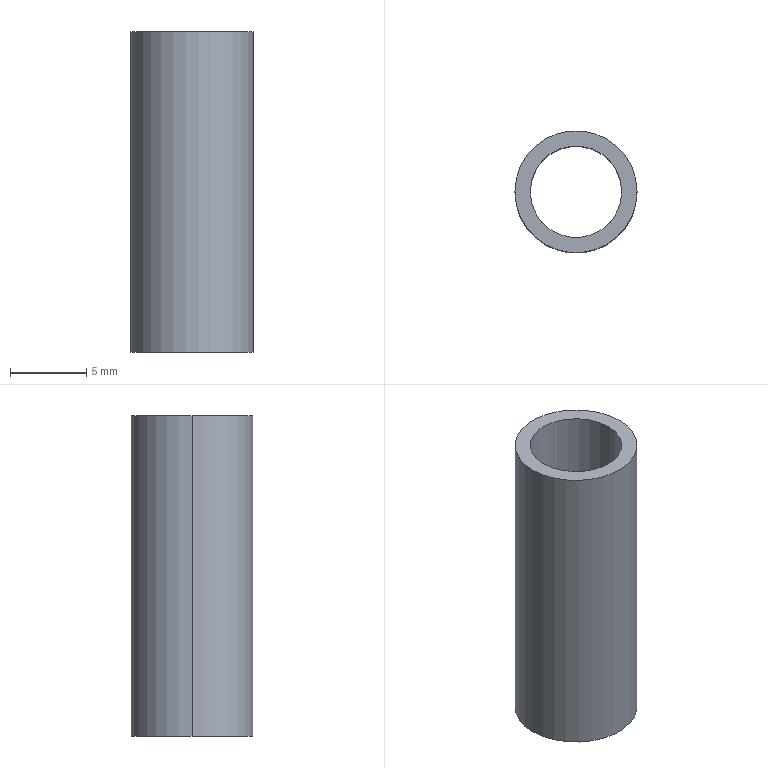Part | STEP file | PN_0001 Wheel body | 1 solid | 6 faces | box 8 x 8 x 21 mm | volume 461.814 mm3 | cylinder 4 | plane 2 | commonest cylinder face diameters 6 x2 8 x2
STEP:
#1=CARTESIAN_POINT('',(0.,0.,0.));
#2=DIRECTION('',(0.,0.,1.));
#3=DIRECTION('',(1.,0.,0.));
#4=AXIS2_PLACEMENT_3D('',#1,#2,#3);
#5=CARTESIAN_POINT('',(20.,-37.5,10.5));
#6=VERTEX_POINT('',#5);
#7=CARTESIAN_POINT('',(20.,-37.5,-10.5));
#8=VERTEX_POINT('',#7);
#9=CARTESIAN_POINT('',(20.,-37.5,10.5));
#10=DIRECTION('',(0.,0.,-1.));
#11=VECTOR('',#10,1.);
#12=LINE('',#9,#11);
#13=CARTESIAN_POINT('',(23.,-37.5,10.5));
#14=DIRECTION('',(0.,0.,-1.));
#15=DIRECTION('',(-1.,0.,0.));
#16=AXIS2_PLACEMENT_3D('',#13,#14,#15);
#17=CYLINDRICAL_SURFACE('',#16,3.);
#18=CARTESIAN_POINT('',(6.283,0.));
#19=DIRECTION('',(0.,1.));
#20=VECTOR('',#19,1.);
#21=LINE('',#18,#20);
#22=(GEOMETRIC_REPRESENTATION_CONTEXT(2)PARAMETRIC_REPRESENTATION_CONTEXT()REPRESENTATION_CONTEXT('',''));
#23=DEFINITIONAL_REPRESENTATION('',(#21),#22);
#24=PCURVE('',#17,#23);
#25=CARTESIAN_POINT('',(23.,-37.5,10.5));
#26=DIRECTION('',(0.,0.,-1.));
#27=DIRECTION('',(-1.,0.,0.));
#28=AXIS2_PLACEMENT_3D('',#25,#26,#27);
#29=CYLINDRICAL_SURFACE('',#28,3.);
#30=CARTESIAN_POINT('',(0.,0.));
#31=DIRECTION('',(0.,1.));
#32=VECTOR('',#31,1.);
#33=LINE('',#30,#32);
#34=(GEOMETRIC_REPRESENTATION_CONTEXT(2)PARAMETRIC_REPRESENTATION_CONTEXT()REPRESENTATION_CONTEXT('',''));
#35=DEFINITIONAL_REPRESENTATION('',(#33),#34);
#36=PCURVE('',#29,#35);
#37=SURFACE_CURVE('',#12,(#24,#36),.PCURVE_S1.);
#38=EDGE_CURVE('',#6,#8,#37,.T.);
#39=ORIENTED_EDGE('',*,*,#38,.T.);
#40=CARTESIAN_POINT('',(26.,-37.5,-10.5));
#41=VERTEX_POINT('',#40);
#42=CARTESIAN_POINT('',(23.,-37.5,-10.5));
#43=DIRECTION('',(0.,0.,1.));
#44=DIRECTION('',(1.,0.,0.));
#45=AXIS2_PLACEMENT_3D('',#42,#43,#44);
#46=CIRCLE('',#45,3.);
#47=CARTESIAN_POINT('',(9.425,21.));
#48=DIRECTION('',(-1.,0.));
#49=VECTOR('',#48,1.);
#50=LINE('',#47,#49);
#51=(GEOMETRIC_REPRESENTATION_CONTEXT(2)PARAMETRIC_REPRESENTATION_CONTEXT()REPRESENTATION_CONTEXT('',''));
#52=DEFINITIONAL_REPRESENTATION('',(#50),#51);
#53=PCURVE('',#17,#52);
#54=CARTESIAN_POINT('',(23.,-37.5,-10.5));
#55=DIRECTION('',(0.,0.,1.));
#56=DIRECTION('',(1.,0.,0.));
#57=AXIS2_PLACEMENT_3D('',#54,#55,#56);
#58=PLANE('',#57);
#59=CARTESIAN_POINT('',(0.,0.));
#60=DIRECTION('',(1.,0.));
#61=AXIS2_PLACEMENT_2D('',#59,#60);
#62=CIRCLE('',#61,3.);
#63=(GEOMETRIC_REPRESENTATION_CONTEXT(2)PARAMETRIC_REPRESENTATION_CONTEXT()REPRESENTATION_CONTEXT('',''));
#64=DEFINITIONAL_REPRESENTATION('',(#62),#63);
#65=PCURVE('',#58,#64);
#66=SURFACE_CURVE('',#46,(#53,#65),.PCURVE_S1.);
#67=EDGE_CURVE('',#8,#41,#66,.T.);
#68=ORIENTED_EDGE('',*,*,#67,.T.);
#69=CARTESIAN_POINT('',(26.,-37.5,10.5));
#70=VERTEX_POINT('',#69);
#71=CARTESIAN_POINT('',(26.,-37.5,10.5));
#72=DIRECTION('',(0.,0.,-1.));
#73=VECTOR('',#72,1.);
#74=LINE('',#71,#73);
#75=CARTESIAN_POINT('',(3.142,0.));
#76=DIRECTION('',(0.,1.));
#77=VECTOR('',#76,1.);
#78=LINE('',#75,#77);
#79=(GEOMETRIC_REPRESENTATION_CONTEXT(2)PARAMETRIC_REPRESENTATION_CONTEXT()REPRESENTATION_CONTEXT('',''));
#80=DEFINITIONAL_REPRESENTATION('',(#78),#79);
#81=PCURVE('',#17,#80);
#82=CARTESIAN_POINT('',(3.142,0.));
#83=DIRECTION('',(0.,1.));
#84=VECTOR('',#83,1.);
#85=LINE('',#82,#84);
#86=(GEOMETRIC_REPRESENTATION_CONTEXT(2)PARAMETRIC_REPRESENTATION_CONTEXT()REPRESENTATION_CONTEXT('',''));
#87=DEFINITIONAL_REPRESENTATION('',(#85),#86);
#88=PCURVE('',#29,#87);
#89=SURFACE_CURVE('',#74,(#81,#88),.PCURVE_S1.);
#90=EDGE_CURVE('',#70,#41,#89,.T.);
#91=ORIENTED_EDGE('',*,*,#90,.F.);
#92=CARTESIAN_POINT('',(23.,-37.5,10.5));
#93=DIRECTION('',(0.,0.,1.));
#94=DIRECTION('',(1.,0.,0.));
#95=AXIS2_PLACEMENT_3D('',#92,#93,#94);
#96=CIRCLE('',#95,3.);
#97=CARTESIAN_POINT('',(9.425,0.));
#98=DIRECTION('',(-1.,0.));
#99=VECTOR('',#98,1.);
#100=LINE('',#97,#99);
#101=(GEOMETRIC_REPRESENTATION_CONTEXT(2)PARAMETRIC_REPRESENTATION_CONTEXT()REPRESENTATION_CONTEXT('',''));
#102=DEFINITIONAL_REPRESENTATION('',(#100),#101);
#103=PCURVE('',#17,#102);
#104=CARTESIAN_POINT('',(23.,-37.5,10.5));
#105=DIRECTION('',(0.,0.,1.));
#106=DIRECTION('',(1.,0.,0.));
#107=AXIS2_PLACEMENT_3D('',#104,#105,#106);
#108=PLANE('',#107);
#109=CARTESIAN_POINT('',(0.,0.));
#110=DIRECTION('',(1.,0.));
#111=AXIS2_PLACEMENT_2D('',#109,#110);
#112=CIRCLE('',#111,3.);
#113=(GEOMETRIC_REPRESENTATION_CONTEXT(2)PARAMETRIC_REPRESENTATION_CONTEXT()REPRESENTATION_CONTEXT('',''));
#114=DEFINITIONAL_REPRESENTATION('',(#112),#113);
#115=PCURVE('',#108,#114);
#116=SURFACE_CURVE('',#96,(#103,#115),.PCURVE_S1.);
#117=EDGE_CURVE('',#6,#70,#116,.T.);
#118=ORIENTED_EDGE('',*,*,#117,.F.);
#119=EDGE_LOOP('',(#39,#68,#91,#118));
#120=FACE_BOUND('',#119,.F.);
#121=ADVANCED_FACE('',(#120),#17,.F.);
#122=CARTESIAN_POINT('',(27.,-37.5,10.5));
#123=VERTEX_POINT('',#122);
#124=CARTESIAN_POINT('',(19.,-37.5,10.5));
#125=VERTEX_POINT('',#124);
#126=CARTESIAN_POINT('',(23.,-37.5,10.5));
#127=DIRECTION('',(0.,0.,1.));
#128=DIRECTION('',(1.,0.,0.));
#129=AXIS2_PLACEMENT_3D('',#126,#127,#128);
#130=CIRCLE('',#129,4.);
#131=CARTESIAN_POINT('',(23.,-37.5,10.5));
#132=DIRECTION('',(0.,0.,-1.));
#133=DIRECTION('',(-1.,0.,0.));
#134=AXIS2_PLACEMENT_3D('',#131,#132,#133);
#135=CYLINDRICAL_SURFACE('',#134,4.);
#136=CARTESIAN_POINT('',(3.142,0.));
#137=DIRECTION('',(-1.,0.));
#138=VECTOR('',#137,1.);
#139=LINE('',#136,#138);
#140=(GEOMETRIC_REPRESENTATION_CONTEXT(2)PARAMETRIC_REPRESENTATION_CONTEXT()REPRESENTATION_CONTEXT('',''));
#141=DEFINITIONAL_REPRESENTATION('',(#139),#140);
#142=PCURVE('',#135,#141);
#143=CARTESIAN_POINT('',(0.,0.));
#144=DIRECTION('',(1.,0.));
#145=AXIS2_PLACEMENT_2D('',#143,#144);
#146=CIRCLE('',#145,4.);
#147=(GEOMETRIC_REPRESENTATION_CONTEXT(2)PARAMETRIC_REPRESENTATION_CONTEXT()REPRESENTATION_CONTEXT('',''));
#148=DEFINITIONAL_REPRESENTATION('',(#146),#147);
#149=PCURVE('',#108,#148);
#150=SURFACE_CURVE('',#130,(#142,#149),.PCURVE_S1.);
#151=EDGE_CURVE('',#123,#125,#150,.T.);
#152=ORIENTED_EDGE('',*,*,#151,.F.);
#153=CARTESIAN_POINT('',(27.,-37.5,-10.5));
#154=VERTEX_POINT('',#153);
#155=CARTESIAN_POINT('',(27.,-37.5,10.5));
#156=DIRECTION('',(0.,0.,-1.));
#157=VECTOR('',#156,1.);
#158=LINE('',#155,#157);
#159=CARTESIAN_POINT('',(3.142,0.));
#160=DIRECTION('',(0.,1.));
#161=VECTOR('',#160,1.);
#162=LINE('',#159,#161);
#163=(GEOMETRIC_REPRESENTATION_CONTEXT(2)PARAMETRIC_REPRESENTATION_CONTEXT()REPRESENTATION_CONTEXT('',''));
#164=DEFINITIONAL_REPRESENTATION('',(#162),#163);
#165=PCURVE('',#135,#164);
#166=CARTESIAN_POINT('',(23.,-37.5,10.5));
#167=DIRECTION('',(0.,0.,-1.));
#168=DIRECTION('',(-1.,0.,0.));
#169=AXIS2_PLACEMENT_3D('',#166,#167,#168);
#170=CYLINDRICAL_SURFACE('',#169,4.);
#171=CARTESIAN_POINT('',(3.142,0.));
#172=DIRECTION('',(0.,1.));
#173=VECTOR('',#172,1.);
#174=LINE('',#171,#173);
#175=(GEOMETRIC_REPRESENTATION_CONTEXT(2)PARAMETRIC_REPRESENTATION_CONTEXT()REPRESENTATION_CONTEXT('',''));
#176=DEFINITIONAL_REPRESENTATION('',(#174),#175);
#177=PCURVE('',#170,#176);
#178=SURFACE_CURVE('',#158,(#165,#177),.PCURVE_S1.);
#179=EDGE_CURVE('',#123,#154,#178,.T.);
#180=ORIENTED_EDGE('',*,*,#179,.T.);
#181=CARTESIAN_POINT('',(19.,-37.5,-10.5));
#182=VERTEX_POINT('',#181);
#183=CARTESIAN_POINT('',(23.,-37.5,-10.5));
#184=DIRECTION('',(0.,0.,1.));
#185=DIRECTION('',(1.,0.,0.));
#186=AXIS2_PLACEMENT_3D('',#183,#184,#185);
#187=CIRCLE('',#186,4.);
#188=CARTESIAN_POINT('',(3.142,21.));
#189=DIRECTION('',(-1.,0.));
#190=VECTOR('',#189,1.);
#191=LINE('',#188,#190);
#192=(GEOMETRIC_REPRESENTATION_CONTEXT(2)PARAMETRIC_REPRESENTATION_CONTEXT()REPRESENTATION_CONTEXT('',''));
#193=DEFINITIONAL_REPRESENTATION('',(#191),#192);
#194=PCURVE('',#135,#193);
#195=CARTESIAN_POINT('',(0.,0.));
#196=DIRECTION('',(1.,0.));
#197=AXIS2_PLACEMENT_2D('',#195,#196);
#198=CIRCLE('',#197,4.);
#199=(GEOMETRIC_REPRESENTATION_CONTEXT(2)PARAMETRIC_REPRESENTATION_CONTEXT()REPRESENTATION_CONTEXT('',''));
#200=DEFINITIONAL_REPRESENTATION('',(#198),#199);
#201=PCURVE('',#58,#200);
#202=SURFACE_CURVE('',#187,(#194,#201),.PCURVE_S1.);
#203=EDGE_CURVE('',#154,#182,#202,.T.);
#204=ORIENTED_EDGE('',*,*,#203,.T.);
#205=CARTESIAN_POINT('',(19.,-37.5,10.5));
#206=DIRECTION('',(0.,0.,-1.));
#207=VECTOR('',#206,1.);
#208=LINE('',#205,#207);
#209=CARTESIAN_POINT('',(0.,0.));
#210=DIRECTION('',(0.,1.));
#211=VECTOR('',#210,1.);
#212=LINE('',#209,#211);
#213=(GEOMETRIC_REPRESENTATION_CONTEXT(2)PARAMETRIC_REPRESENTATION_CONTEXT()REPRESENTATION_CONTEXT('',''));
#214=DEFINITIONAL_REPRESENTATION('',(#212),#213);
#215=PCURVE('',#135,#214);
#216=CARTESIAN_POINT('',(6.283,0.));
#217=DIRECTION('',(0.,1.));
#218=VECTOR('',#217,1.);
#219=LINE('',#216,#218);
#220=(GEOMETRIC_REPRESENTATION_CONTEXT(2)PARAMETRIC_REPRESENTATION_CONTEXT()REPRESENTATION_CONTEXT('',''));
#221=DEFINITIONAL_REPRESENTATION('',(#219),#220);
#222=PCURVE('',#170,#221);
#223=SURFACE_CURVE('',#208,(#215,#222),.PCURVE_S1.);
#224=EDGE_CURVE('',#125,#182,#223,.T.);
#225=ORIENTED_EDGE('',*,*,#224,.F.);
#226=EDGE_LOOP('',(#152,#180,#204,#225));
#227=FACE_BOUND('',#226,.T.);
#228=ADVANCED_FACE('',(#227),#135,.T.);
#229=CARTESIAN_POINT('',(23.,-37.5,10.5));
#230=DIRECTION('',(0.,0.,1.));
#231=DIRECTION('',(1.,0.,0.));
#232=AXIS2_PLACEMENT_3D('',#229,#230,#231);
#233=CIRCLE('',#232,4.);
#234=CARTESIAN_POINT('',(0.,0.));
#235=DIRECTION('',(1.,0.));
#236=AXIS2_PLACEMENT_2D('',#234,#235);
#237=CIRCLE('',#236,4.);
#238=(GEOMETRIC_REPRESENTATION_CONTEXT(2)PARAMETRIC_REPRESENTATION_CONTEXT()REPRESENTATION_CONTEXT('',''));
#239=DEFINITIONAL_REPRESENTATION('',(#237),#238);
#240=PCURVE('',#108,#239);
#241=CARTESIAN_POINT('',(9.425,0.));
#242=DIRECTION('',(-1.,0.));
#243=VECTOR('',#242,1.);
#244=LINE('',#241,#243);
#245=(GEOMETRIC_REPRESENTATION_CONTEXT(2)PARAMETRIC_REPRESENTATION_CONTEXT()REPRESENTATION_CONTEXT('',''));
#246=DEFINITIONAL_REPRESENTATION('',(#244),#245);
#247=PCURVE('',#170,#246);
#248=SURFACE_CURVE('',#233,(#240,#247),.PCURVE_S1.);
#249=EDGE_CURVE('',#125,#123,#248,.T.);
#250=ORIENTED_EDGE('',*,*,#249,.T.);
#251=ORIENTED_EDGE('',*,*,#151,.T.);
#252=EDGE_LOOP('',(#250,#251));
#253=FACE_BOUND('',#252,.T.);
#254=ORIENTED_EDGE('',*,*,#117,.F.);
#255=CARTESIAN_POINT('',(23.,-37.5,10.5));
#256=DIRECTION('',(0.,0.,1.));
#257=DIRECTION('',(1.,0.,0.));
#258=AXIS2_PLACEMENT_3D('',#255,#256,#257);
#259=CIRCLE('',#258,3.);
#260=CARTESIAN_POINT('',(0.,0.));
#261=DIRECTION('',(1.,0.));
#262=AXIS2_PLACEMENT_2D('',#260,#261);
#263=CIRCLE('',#262,3.);
#264=(GEOMETRIC_REPRESENTATION_CONTEXT(2)PARAMETRIC_REPRESENTATION_CONTEXT()REPRESENTATION_CONTEXT('',''));
#265=DEFINITIONAL_REPRESENTATION('',(#263),#264);
#266=PCURVE('',#108,#265);
#267=CARTESIAN_POINT('',(3.142,0.));
#268=DIRECTION('',(-1.,0.));
#269=VECTOR('',#268,1.);
#270=LINE('',#267,#269);
#271=(GEOMETRIC_REPRESENTATION_CONTEXT(2)PARAMETRIC_REPRESENTATION_CONTEXT()REPRESENTATION_CONTEXT('',''));
#272=DEFINITIONAL_REPRESENTATION('',(#270),#271);
#273=PCURVE('',#29,#272);
#274=SURFACE_CURVE('',#259,(#266,#273),.PCURVE_S1.);
#275=EDGE_CURVE('',#70,#6,#274,.T.);
#276=ORIENTED_EDGE('',*,*,#275,.F.);
#277=EDGE_LOOP('',(#254,#276));
#278=FACE_BOUND('',#277,.T.);
#279=ADVANCED_FACE('',(#253,#278),#108,.T.);
#280=CARTESIAN_POINT('',(23.,-37.5,-10.5));
#281=DIRECTION('',(0.,0.,1.));
#282=DIRECTION('',(1.,0.,0.));
#283=AXIS2_PLACEMENT_3D('',#280,#281,#282);
#284=CIRCLE('',#283,4.);
#285=CARTESIAN_POINT('',(0.,0.));
#286=DIRECTION('',(1.,0.));
#287=AXIS2_PLACEMENT_2D('',#285,#286);
#288=CIRCLE('',#287,4.);
#289=(GEOMETRIC_REPRESENTATION_CONTEXT(2)PARAMETRIC_REPRESENTATION_CONTEXT()REPRESENTATION_CONTEXT('',''));
#290=DEFINITIONAL_REPRESENTATION('',(#288),#289);
#291=PCURVE('',#58,#290);
#292=CARTESIAN_POINT('',(9.425,21.));
#293=DIRECTION('',(-1.,0.));
#294=VECTOR('',#293,1.);
#295=LINE('',#292,#294);
#296=(GEOMETRIC_REPRESENTATION_CONTEXT(2)PARAMETRIC_REPRESENTATION_CONTEXT()REPRESENTATION_CONTEXT('',''));
#297=DEFINITIONAL_REPRESENTATION('',(#295),#296);
#298=PCURVE('',#170,#297);
#299=SURFACE_CURVE('',#284,(#291,#298),.PCURVE_S1.);
#300=EDGE_CURVE('',#182,#154,#299,.T.);
#301=ORIENTED_EDGE('',*,*,#300,.F.);
#302=ORIENTED_EDGE('',*,*,#203,.F.);
#303=EDGE_LOOP('',(#301,#302));
#304=FACE_BOUND('',#303,.T.);
#305=ORIENTED_EDGE('',*,*,#67,.T.);
#306=CARTESIAN_POINT('',(23.,-37.5,-10.5));
#307=DIRECTION('',(0.,0.,1.));
#308=DIRECTION('',(1.,0.,0.));
#309=AXIS2_PLACEMENT_3D('',#306,#307,#308);
#310=CIRCLE('',#309,3.);
#311=CARTESIAN_POINT('',(0.,0.));
#312=DIRECTION('',(1.,0.));
#313=AXIS2_PLACEMENT_2D('',#311,#312);
#314=CIRCLE('',#313,3.);
#315=(GEOMETRIC_REPRESENTATION_CONTEXT(2)PARAMETRIC_REPRESENTATION_CONTEXT()REPRESENTATION_CONTEXT('',''));
#316=DEFINITIONAL_REPRESENTATION('',(#314),#315);
#317=PCURVE('',#58,#316);
#318=CARTESIAN_POINT('',(3.142,21.));
#319=DIRECTION('',(-1.,0.));
#320=VECTOR('',#319,1.);
#321=LINE('',#318,#320);
#322=(GEOMETRIC_REPRESENTATION_CONTEXT(2)PARAMETRIC_REPRESENTATION_CONTEXT()REPRESENTATION_CONTEXT('',''));
#323=DEFINITIONAL_REPRESENTATION('',(#321),#322);
#324=PCURVE('',#29,#323);
#325=SURFACE_CURVE('',#310,(#317,#324),.PCURVE_S1.);
#326=EDGE_CURVE('',#41,#8,#325,.T.);
#327=ORIENTED_EDGE('',*,*,#326,.T.);
#328=EDGE_LOOP('',(#305,#327));
#329=FACE_BOUND('',#328,.T.);
#330=ADVANCED_FACE('',(#304,#329),#58,.F.);
#331=ORIENTED_EDGE('',*,*,#179,.F.);
#332=ORIENTED_EDGE('',*,*,#249,.F.);
#333=ORIENTED_EDGE('',*,*,#224,.T.);
#334=ORIENTED_EDGE('',*,*,#300,.T.);
#335=EDGE_LOOP('',(#331,#332,#333,#334));
#336=FACE_BOUND('',#335,.T.);
#337=ADVANCED_FACE('',(#336),#170,.T.);
#338=ORIENTED_EDGE('',*,*,#326,.T.);
#339=ORIENTED_EDGE('',*,*,#38,.F.);
#340=ORIENTED_EDGE('',*,*,#275,.F.);
#341=ORIENTED_EDGE('',*,*,#90,.T.);
#342=EDGE_LOOP('',(#338,#339,#340,#341));
#343=FACE_BOUND('',#342,.F.);
#344=ADVANCED_FACE('',(#343),#29,.F.);
#345=CLOSED_SHELL('',(#121,#228,#279,#330,#337,#344));
#346=MANIFOLD_SOLID_BREP('',#345);
#347=(LENGTH_UNIT()NAMED_UNIT(*)SI_UNIT(.MILLI.,.METRE.));
#348=UNCERTAINTY_MEASURE_WITH_UNIT(LENGTH_MEASURE(0.0000001),#347,'','');
#349=(NAMED_UNIT(*)PLANE_ANGLE_UNIT()SI_UNIT($,.RADIAN.));
#350=(NAMED_UNIT(*)SI_UNIT($,.STERADIAN.)SOLID_ANGLE_UNIT());
#351=(GEOMETRIC_REPRESENTATION_CONTEXT(3)GLOBAL_UNCERTAINTY_ASSIGNED_CONTEXT((#348))GLOBAL_UNIT_ASSIGNED_CONTEXT((#347,#349,#350))REPRESENTATION_CONTEXT('',''));
#352=ADVANCED_BREP_SHAPE_REPRESENTATION('',(#4,#346),#351);